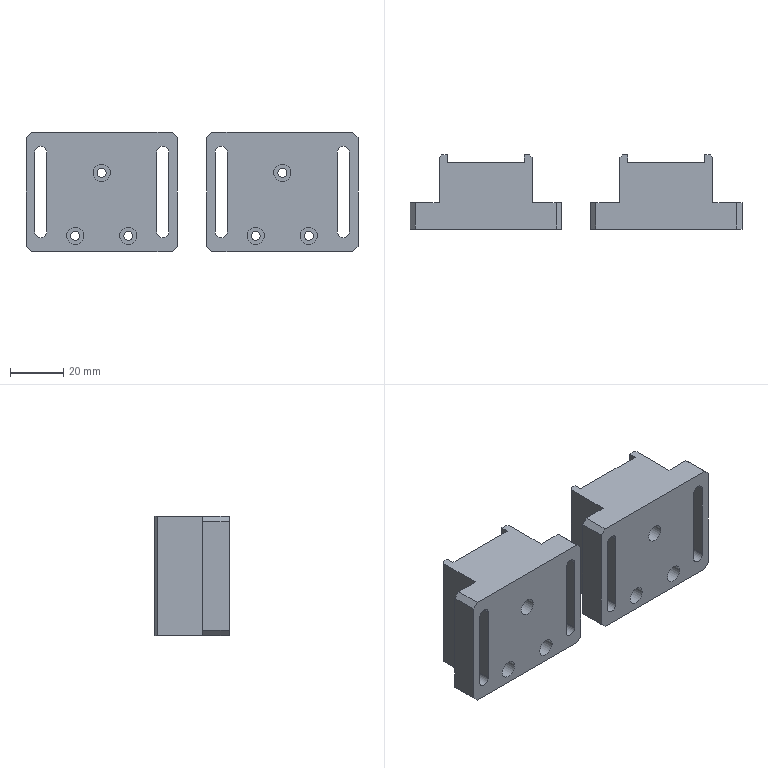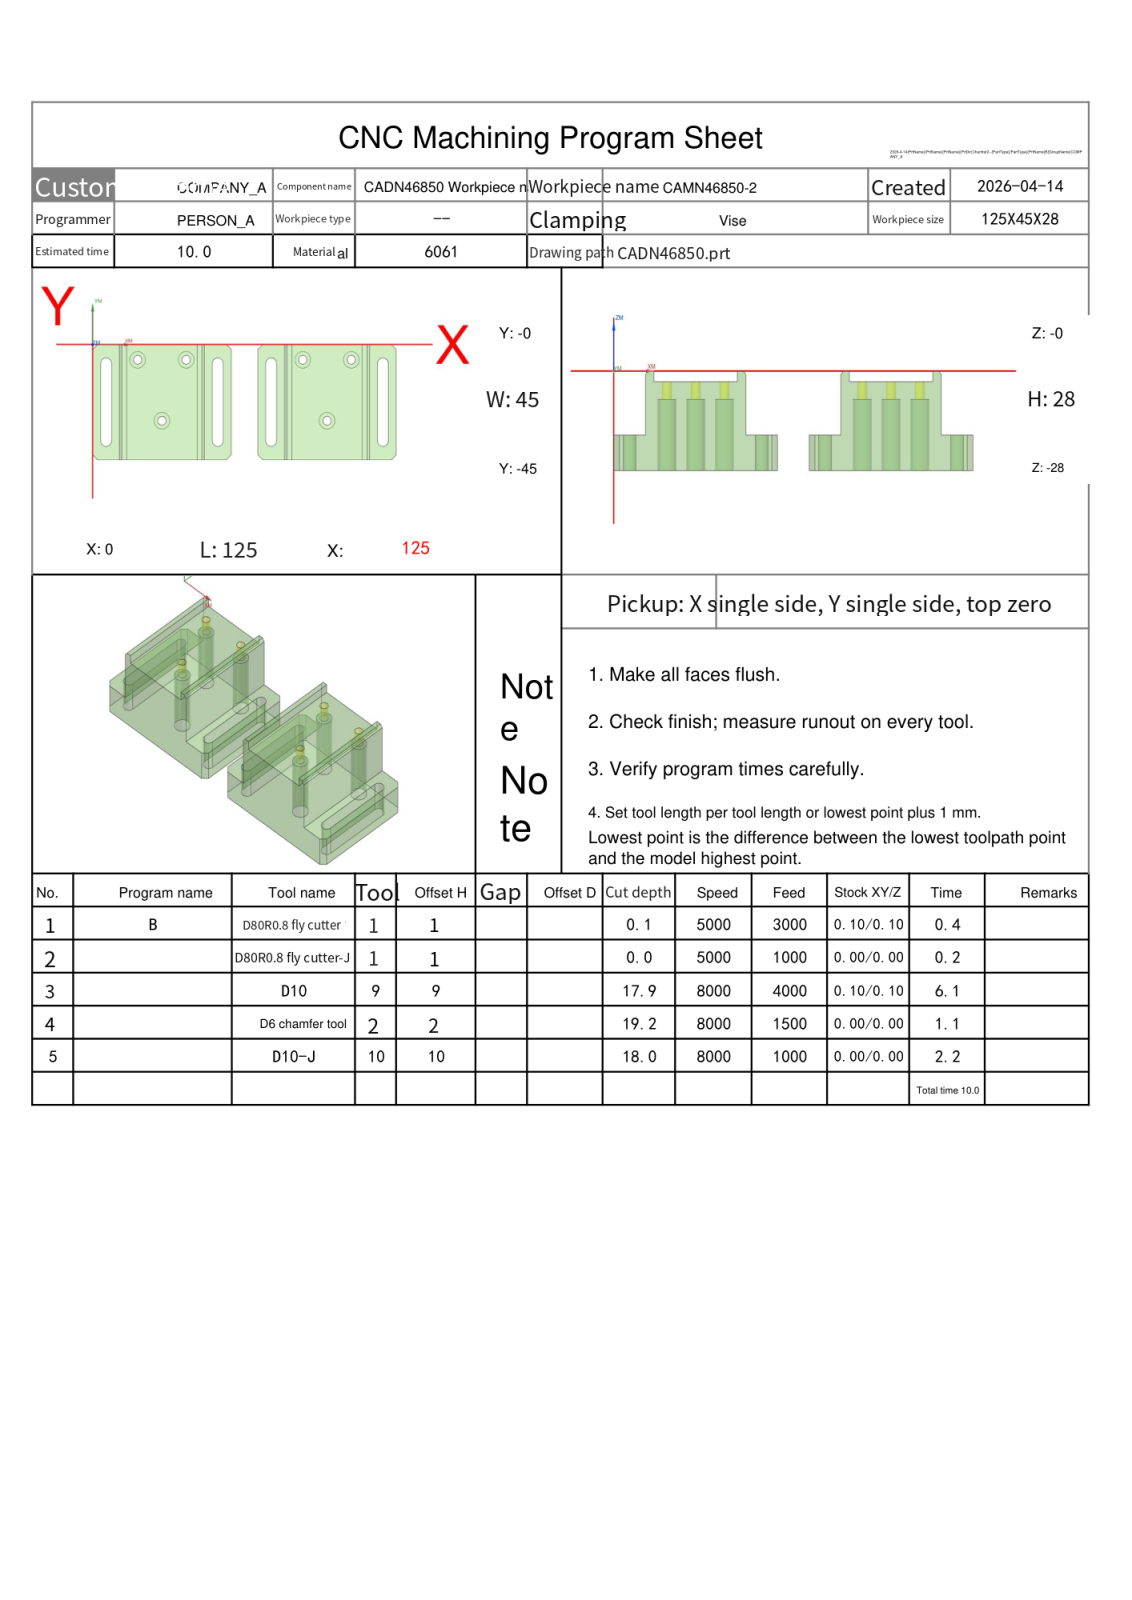NC program | NX | posted by the shop | part box 125 x 28 x 45 mm
Lines 3147 to 3399 of 3399:
N5 T10 M06
(D10-J  D=10. R=0. H=10 ce=0.40 di=0.00)
G00 G90 G54 X21.401 Y-52. M03 S8000
G43 H10 Z11.8
M08
Z-1.5
G01 Z-3. F1000.
Y-48.
G03 X19.401 Y-50. I0.0 J-2.
G01 Y4.1
G02 X20.301 Y5. I.9 J0.0
G01 X22.951
G02 X23.951 Y4. I0.0 J-1.
G01 Y-49.1
G03 X24.851 Y-50. I.9 J0.0
G01 X27.5
G03 X28.5 Y-49. I0.0 J1.
G01 Y4.1
G02 X29.4 Y5. I.9 J0.0
G01 X32.05
G02 X33.05 Y4. I0.0 J-1.
G01 Y-49.1
G03 X33.95 Y-50. I.9 J0.0
G01 X36.6
G03 X37.6 Y-49. I0.0 J1.
G01 Y5.
G03 X35.6 Y7. I-2. J0.0
G01 Z-1.5
G00 Z3.
X89.401 Y-52.
Z-1.5
G01 Z-3.
Y-48.
G03 X87.401 Y-50. I0.0 J-2.
G01 Y4.1
G02 X88.301 Y5. I.9 J0.0
G01 X90.951
G02 X91.951 Y4. I0.0 J-1.
G01 Y-49.1
G03 X92.851 Y-50. I.9 J0.0
G01 X95.5
G03 X96.5 Y-49. I0.0 J1.
G01 Y4.1
G02 X97.4 Y5. I.9 J0.0
G01 X100.05
G02 X101.05 Y4. I0.0 J-1.
G01 Y-49.1
G03 X101.95 Y-50. I.9 J0.0
G01 X104.6
G03 X105.6 Y-49. I0.0 J1.
G01 Y5.
G03 X103.6 Y7. I-2. J0.0
G01 Z-1.5
G00 Z11.8
G00 G90 X127.062 Y5.837 M03 S8000
Z11.8
Z-16.5
G01 Z-18. F1000.
G03 X126. Y4.071 I.938 J-1.766
G01 Y-48.657
G02 X125.708 Y-49.364 I-1. J.001
G01 X125.364 Y-49.707
G02 X124.657 Y-50. I-.707 J.707
G01 X123.699
G02 X122.7 Y-49.001 I.001 J1.
G01 Y4.1
G03 X121.8 Y5. I-.9 J0.0
G01 X120.4
G03 X119.4 Y4. I0.0 J-1.
G01 Y-50.
G03 X121.4 Y-52. I2. J0.0
G01 Z-16.5
G00 Z3.
X53.401
Z-16.5
G01 Z-18.
Y-48.
G03 X51.401 Y-50. I0.0 J-2.
G01 Y4.
G02 X52.401 Y5. I1. J0.0
G01 X54.941
G02 X55.841 Y4.1 I0.0 J-.9
G01 Y-49.001
G03 X56.84 Y-50. I1. J.001
G01 X57.005
X57.137 Y-49.991
X59.414 Y-49.686
G03 X60.281 Y-48.695 I-.133 J.991
G01 Y3.57
G02 X61.281 Y4.57 I1. J0.0
G01 X63.82
G02 X64.72 Y3.67 I0.0 J-.9
G01 Y-48.695
G03 X65.587 Y-49.686 I1. J.001
G01 X67.863 Y-49.991
X67.995 Y-50.
X68.161
G03 X69.16 Y-49.001 I-.001 J1.
G01 Y4.1
G02 X70.06 Y5. I.9 J0.0
G01 X72.6
G02 X73.6 Y4. I0.0 J-1.
G01 Y-50.
G02 X71.6 Y-52. I-2. J0.0
G01 Z-16.5
G00 Z3.
X-2.062 Y-50.837
Z-16.5
G01 Z-18.
G03 X-1. Y-49.071 I-.938 J1.766
G01 Y3.657
G02 X-.707 Y4.364 I1. J-.001
G01 X-.364 Y4.707
G02 X.343 Y5. I.707 J-.707
G01 X1.301
G02 X2.3 Y4.001 I-.001 J-1.
G01 Y-49.1
G03 X3.2 Y-50. I.9 J0.0
G01 X4.6
G03 X5.6 Y-49. I0.0 J1.
G01 Y5.
G03 X3.6 Y7. I-2. J0.0
G01 Z-16.5
G00 Z11.8
G00 G90 X121.199 Y7. M03 S8000
Z11.8
Z-8.
G01 Z-9. F1000.
G41 D10
X120.999
G03 X119. Y5. I.001 J-2.
G01 Y-50.
G03 X120.999 Y-52. I2. J0.0
G01 G40 X121.199
Z-8.
G00 Y7.
Z-17.
G01 Z-18.
G41 D10
X120.999
G03 X119. Y5. I.001 J-2.
G01 Y-50.
G03 X120.999 Y-52. I2. J0.0
G01 G40 X121.199
Z-17.
G00 Z3.
X71.801
Z-8.
G01 Z-9.
G41 D10
X72.001
G03 X74. Y-50. I-.001 J2.
G01 Y5.
G03 X72.001 Y7. I-2. J0.0
G01 G40 X71.801
Z-8.
G00 X53.199
G01 Z-9.
G41 D10
X52.999
G03 X51. Y5. I.001 J-2.
G01 Y-50.
G03 X52.999 Y-52. I2. J0.0
G01 G40 X53.199
Z-8.
G00 X71.801
Z-17.
G01 Z-18.
G41 D10
X72.001
G03 X74. Y-50. I-.001 J2.
G01 Y5.
G03 X72.001 Y7. I-2. J0.0
G01 G40 X71.801
Z-17.
G00 X53.199
G01 Z-18.
G41 D10
X52.999
G03 X51. Y5. I.001 J-2.
G01 Y-50.
G03 X52.999 Y-52. I2. J0.0
G01 G40 X53.199
Z-17.
G00 Z3.
X3.801
Z-8.
G01 Z-9.
G41 D10
X4.001
G03 X6. Y-50. I-.001 J2.
G01 Y5.
G03 X4.001 Y7. I-2. J0.0
G01 G40 X3.801
Z-8.
G00 Y-52.
Z-17.
G01 Z-18.
G41 D10
X4.001
G03 X6. Y-50. I-.001 J2.
G01 Y5.
G03 X4.001 Y7. I-2. J0.0
G01 G40 X3.801
Z-17.
G00 Z11.8
G00 G90 X20.857 Y7.007 M03 S8000
Z11.8
Z-2.
G01 Z-3. F1000.
G41 D10
X20.66 Y6.975
G03 X18.975 Y5. I.315 J-1.975
G01 Y-50.
G03 X20.66 Y-51.975 I2. J0.0
G01 G40 X20.857 Y-52.007
Z-2.
G00 X36.143
G01 Z-3.
G41 D10
X36.34 Y-51.975
G03 X38.025 Y-50. I-.315 J1.975
G01 Y5.
G03 X36.34 Y6.975 I-2. J0.0
G01 G40 X36.143 Y7.007
Z-2.
G00 Z3.
X88.857
Z-2.
G01 Z-3.
G41 D10
X88.66 Y6.975
G03 X86.975 Y5. I.315 J-1.975
G01 Y-50.
G03 X88.66 Y-51.975 I2. J0.0
G01 G40 X88.857 Y-52.007
Z-2.
G00 X104.143
G01 Z-3.
G41 D10
X104.34 Y-51.975
G03 X106.025 Y-50. I-.315 J1.975
G01 Y5.
G03 X104.34 Y6.975 I-2. J0.0
G01 G40 X104.143 Y7.007
Z-2.
G00 Z11.8
M05
M09
G91 G28 Z0.0
G91 G28 Y0.0
M30
%